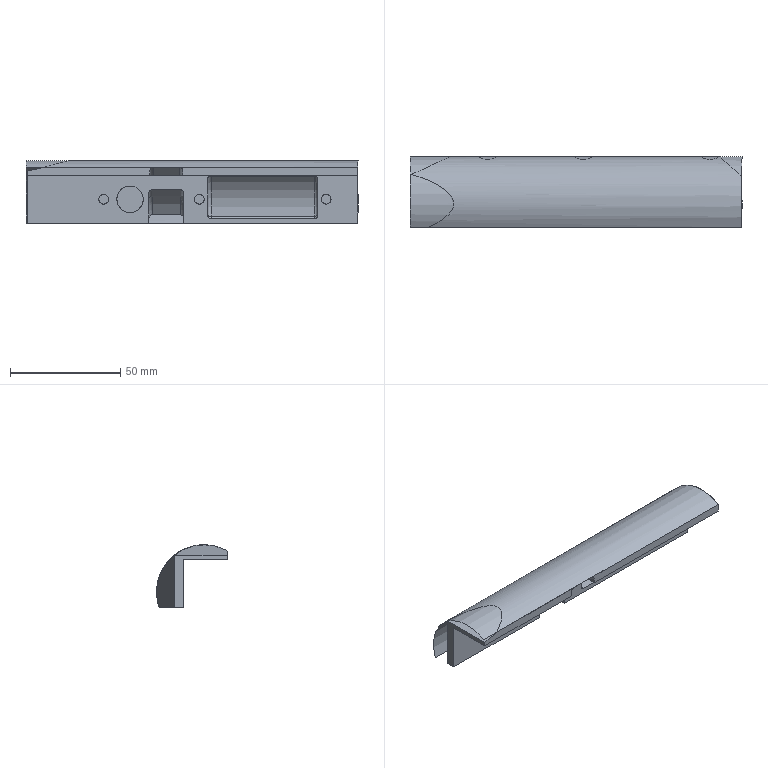Part | 1 solid | 65 faces | volume 77278 mm3 | cylinder 25 | plane 23 | spline 9 | torus 4 | sphere 4 | commonest cylinder face diameters 3 x8 4.4 x6 7 x6 12 x2 37 x1 43 x1